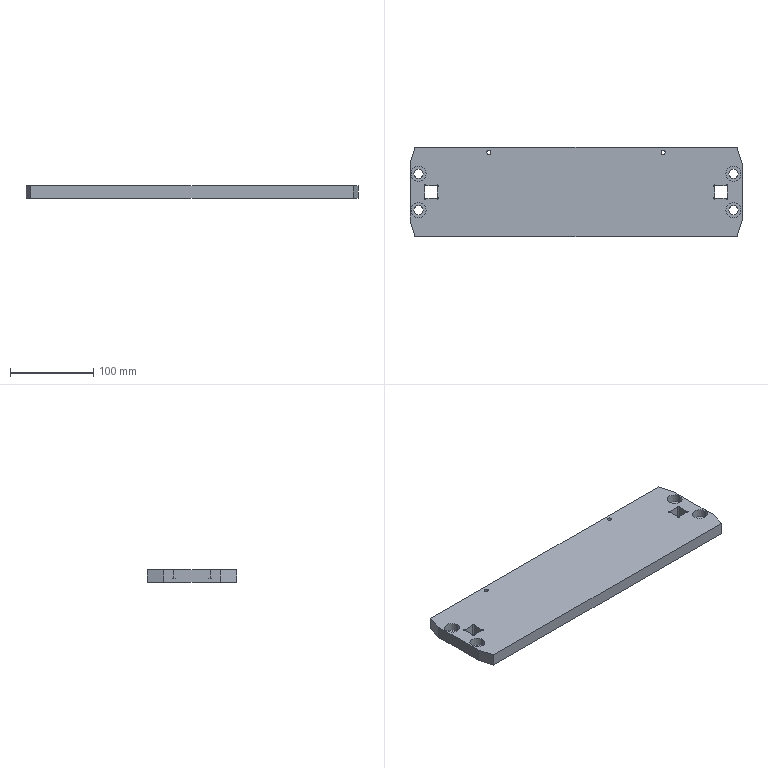Part | STEP file | Column cover plate | 1 solid | 54 faces | box 400 x 107.5 x 15 mm | volume 621699 mm3 | cylinder 32 | plane 22 | commonest cylinder face diameters 2 x12 11 x8 18 x8 5 x4